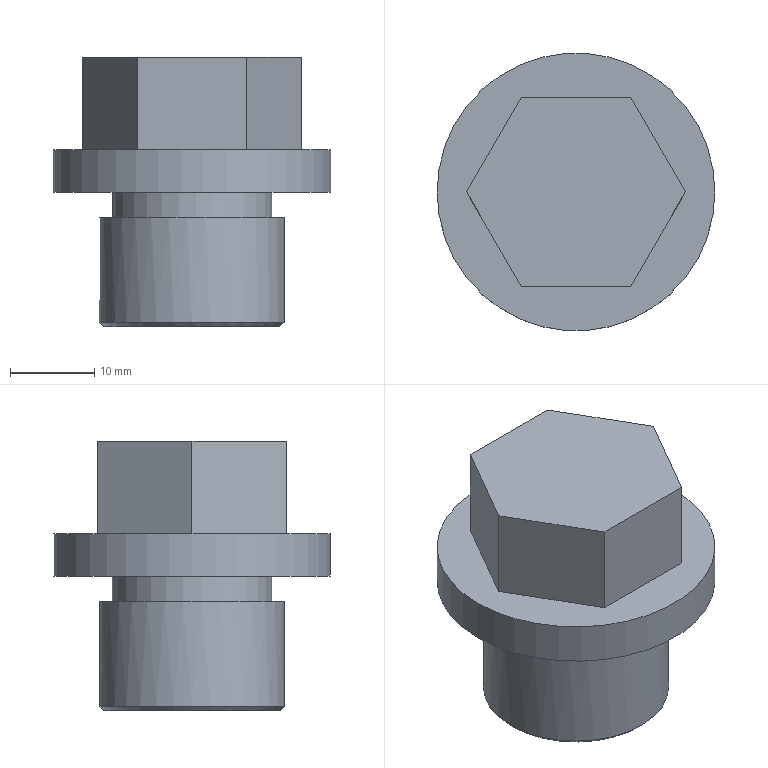Part | NX | features DATUM_CSYS 5, EXTRUDE 4, SKETCH 4, CHAMFER 1 | 1 solid | 15 faces | box 33 x 33 x 32 mm | volume 14890 mm3 | plane 11 | cylinder 3 | cone 1 | commonest cylinder face diameters 19 x1 22 x1 33 x1
STEP:
#1=CARTESIAN_POINT('',(-13.,0.,0.));
#2=VERTEX_POINT('',#1);
#3=CARTESIAN_POINT('',(-6.5,-11.258,0.));
#4=VERTEX_POINT('',#3);
#5=CARTESIAN_POINT('',(-13.,0.,0.));
#6=DIRECTION('',(0.5,-0.866,0.));
#7=VECTOR('',#6,1000.);
#8=LINE('',#5,#7);
#9=EDGE_CURVE('',#2,#4,#8,.T.);
#10=ORIENTED_EDGE('',*,*,#9,.T.);
#11=CARTESIAN_POINT('',(-6.5,-11.258,11.));
#12=VERTEX_POINT('',#11);
#13=CARTESIAN_POINT('',(-6.5,-11.258,11.));
#14=DIRECTION('',(0.,0.,-1.));
#15=VECTOR('',#14,1000.);
#16=LINE('',#13,#15);
#17=EDGE_CURVE('',#12,#4,#16,.T.);
#18=ORIENTED_EDGE('',*,*,#17,.F.);
#19=CARTESIAN_POINT('',(-13.,0.,11.));
#20=VERTEX_POINT('',#19);
#21=CARTESIAN_POINT('',(-13.,0.,11.));
#22=DIRECTION('',(0.5,-0.866,0.));
#23=VECTOR('',#22,1000.);
#24=LINE('',#21,#23);
#25=EDGE_CURVE('',#20,#12,#24,.T.);
#26=ORIENTED_EDGE('',*,*,#25,.F.);
#27=CARTESIAN_POINT('',(-13.,0.,11.));
#28=DIRECTION('',(0.,0.,-1.));
#29=VECTOR('',#28,1000.);
#30=LINE('',#27,#29);
#31=EDGE_CURVE('',#20,#2,#30,.T.);
#32=ORIENTED_EDGE('',*,*,#31,.T.);
#33=EDGE_LOOP('',(#10,#18,#26,#32));
#34=FACE_BOUND('',#33,.T.);
#35=CARTESIAN_POINT('',(-13.,0.,11.));
#36=DIRECTION('',(0.866,0.5,0.));
#37=DIRECTION('',(-0.5,0.866,0.));
#38=AXIS2_PLACEMENT_3D('',#35,#36,#37);
#39=PLANE('',#38);
#40=ADVANCED_FACE('',(#34),#39,.F.);
#41=CARTESIAN_POINT('',(6.5,-11.258,0.));
#42=VERTEX_POINT('',#41);
#43=CARTESIAN_POINT('',(-6.5,-11.258,0.));
#44=DIRECTION('',(1.,0.,0.));
#45=VECTOR('',#44,1000.);
#46=LINE('',#43,#45);
#47=EDGE_CURVE('',#4,#42,#46,.T.);
#48=ORIENTED_EDGE('',*,*,#47,.T.);
#49=CARTESIAN_POINT('',(6.5,-11.258,11.));
#50=VERTEX_POINT('',#49);
#51=CARTESIAN_POINT('',(6.5,-11.258,11.));
#52=DIRECTION('',(0.,0.,-1.));
#53=VECTOR('',#52,1000.);
#54=LINE('',#51,#53);
#55=EDGE_CURVE('',#50,#42,#54,.T.);
#56=ORIENTED_EDGE('',*,*,#55,.F.);
#57=CARTESIAN_POINT('',(-6.5,-11.258,11.));
#58=DIRECTION('',(1.,0.,0.));
#59=VECTOR('',#58,1000.);
#60=LINE('',#57,#59);
#61=EDGE_CURVE('',#12,#50,#60,.T.);
#62=ORIENTED_EDGE('',*,*,#61,.F.);
#63=ORIENTED_EDGE('',*,*,#17,.T.);
#64=EDGE_LOOP('',(#48,#56,#62,#63));
#65=FACE_BOUND('',#64,.T.);
#66=CARTESIAN_POINT('',(-6.5,-11.258,11.));
#67=DIRECTION('',(0.,1.,0.));
#68=DIRECTION('',(-1.,0.,0.));
#69=AXIS2_PLACEMENT_3D('',#66,#67,#68);
#70=PLANE('',#69);
#71=ADVANCED_FACE('',(#65),#70,.F.);
#72=CARTESIAN_POINT('',(13.,0.,0.));
#73=VERTEX_POINT('',#72);
#74=CARTESIAN_POINT('',(6.5,-11.258,0.));
#75=DIRECTION('',(0.5,0.866,0.));
#76=VECTOR('',#75,1000.);
#77=LINE('',#74,#76);
#78=EDGE_CURVE('',#42,#73,#77,.T.);
#79=ORIENTED_EDGE('',*,*,#78,.T.);
#80=CARTESIAN_POINT('',(13.,0.,11.));
#81=VERTEX_POINT('',#80);
#82=CARTESIAN_POINT('',(13.,0.,11.));
#83=DIRECTION('',(0.,0.,-1.));
#84=VECTOR('',#83,1000.);
#85=LINE('',#82,#84);
#86=EDGE_CURVE('',#81,#73,#85,.T.);
#87=ORIENTED_EDGE('',*,*,#86,.F.);
#88=CARTESIAN_POINT('',(6.5,-11.258,11.));
#89=DIRECTION('',(0.5,0.866,0.));
#90=VECTOR('',#89,1000.);
#91=LINE('',#88,#90);
#92=EDGE_CURVE('',#50,#81,#91,.T.);
#93=ORIENTED_EDGE('',*,*,#92,.F.);
#94=ORIENTED_EDGE('',*,*,#55,.T.);
#95=EDGE_LOOP('',(#79,#87,#93,#94));
#96=FACE_BOUND('',#95,.T.);
#97=CARTESIAN_POINT('',(6.5,-11.258,11.));
#98=DIRECTION('',(-0.866,0.5,0.));
#99=DIRECTION('',(-0.5,-0.866,0.));
#100=AXIS2_PLACEMENT_3D('',#97,#98,#99);
#101=PLANE('',#100);
#102=ADVANCED_FACE('',(#96),#101,.F.);
#103=CARTESIAN_POINT('',(6.5,11.258,0.));
#104=VERTEX_POINT('',#103);
#105=CARTESIAN_POINT('',(13.,0.,0.));
#106=DIRECTION('',(-0.5,0.866,0.));
#107=VECTOR('',#106,1000.);
#108=LINE('',#105,#107);
#109=EDGE_CURVE('',#73,#104,#108,.T.);
#110=ORIENTED_EDGE('',*,*,#109,.T.);
#111=CARTESIAN_POINT('',(6.5,11.258,11.));
#112=VERTEX_POINT('',#111);
#113=CARTESIAN_POINT('',(6.5,11.258,11.));
#114=DIRECTION('',(0.,0.,-1.));
#115=VECTOR('',#114,1000.);
#116=LINE('',#113,#115);
#117=EDGE_CURVE('',#112,#104,#116,.T.);
#118=ORIENTED_EDGE('',*,*,#117,.F.);
#119=CARTESIAN_POINT('',(13.,0.,11.));
#120=DIRECTION('',(-0.5,0.866,0.));
#121=VECTOR('',#120,1000.);
#122=LINE('',#119,#121);
#123=EDGE_CURVE('',#81,#112,#122,.T.);
#124=ORIENTED_EDGE('',*,*,#123,.F.);
#125=ORIENTED_EDGE('',*,*,#86,.T.);
#126=EDGE_LOOP('',(#110,#118,#124,#125));
#127=FACE_BOUND('',#126,.T.);
#128=CARTESIAN_POINT('',(13.,0.,11.));
#129=DIRECTION('',(-0.866,-0.5,0.));
#130=DIRECTION('',(0.5,-0.866,0.));
#131=AXIS2_PLACEMENT_3D('',#128,#129,#130);
#132=PLANE('',#131);
#133=ADVANCED_FACE('',(#127),#132,.F.);
#134=CARTESIAN_POINT('',(-6.5,11.258,0.));
#135=VERTEX_POINT('',#134);
#136=CARTESIAN_POINT('',(6.5,11.258,0.));
#137=DIRECTION('',(-1.,0.,0.));
#138=VECTOR('',#137,1000.);
#139=LINE('',#136,#138);
#140=EDGE_CURVE('',#104,#135,#139,.T.);
#141=ORIENTED_EDGE('',*,*,#140,.T.);
#142=CARTESIAN_POINT('',(-6.5,11.258,11.));
#143=VERTEX_POINT('',#142);
#144=CARTESIAN_POINT('',(-6.5,11.258,11.));
#145=DIRECTION('',(0.,0.,-1.));
#146=VECTOR('',#145,1000.);
#147=LINE('',#144,#146);
#148=EDGE_CURVE('',#143,#135,#147,.T.);
#149=ORIENTED_EDGE('',*,*,#148,.F.);
#150=CARTESIAN_POINT('',(6.5,11.258,11.));
#151=DIRECTION('',(-1.,0.,0.));
#152=VECTOR('',#151,1000.);
#153=LINE('',#150,#152);
#154=EDGE_CURVE('',#112,#143,#153,.T.);
#155=ORIENTED_EDGE('',*,*,#154,.F.);
#156=ORIENTED_EDGE('',*,*,#117,.T.);
#157=EDGE_LOOP('',(#141,#149,#155,#156));
#158=FACE_BOUND('',#157,.T.);
#159=CARTESIAN_POINT('',(6.5,11.258,11.));
#160=DIRECTION('',(0.,-1.,0.));
#161=DIRECTION('',(1.,0.,0.));
#162=AXIS2_PLACEMENT_3D('',#159,#160,#161);
#163=PLANE('',#162);
#164=ADVANCED_FACE('',(#158),#163,.F.);
#165=CARTESIAN_POINT('',(-6.5,11.258,0.));
#166=DIRECTION('',(-0.5,-0.866,0.));
#167=VECTOR('',#166,1000.);
#168=LINE('',#165,#167);
#169=EDGE_CURVE('',#135,#2,#168,.T.);
#170=ORIENTED_EDGE('',*,*,#169,.T.);
#171=ORIENTED_EDGE('',*,*,#31,.F.);
#172=CARTESIAN_POINT('',(-6.5,11.258,11.));
#173=DIRECTION('',(-0.5,-0.866,0.));
#174=VECTOR('',#173,1000.);
#175=LINE('',#172,#174);
#176=EDGE_CURVE('',#143,#20,#175,.T.);
#177=ORIENTED_EDGE('',*,*,#176,.F.);
#178=ORIENTED_EDGE('',*,*,#148,.T.);
#179=EDGE_LOOP('',(#170,#171,#177,#178));
#180=FACE_BOUND('',#179,.T.);
#181=CARTESIAN_POINT('',(-6.5,11.258,11.));
#182=DIRECTION('',(0.866,-0.5,0.));
#183=DIRECTION('',(0.5,0.866,0.));
#184=AXIS2_PLACEMENT_3D('',#181,#182,#183);
#185=PLANE('',#184);
#186=ADVANCED_FACE('',(#180),#185,.F.);
#187=ORIENTED_EDGE('',*,*,#25,.T.);
#188=ORIENTED_EDGE('',*,*,#61,.T.);
#189=ORIENTED_EDGE('',*,*,#92,.T.);
#190=ORIENTED_EDGE('',*,*,#123,.T.);
#191=ORIENTED_EDGE('',*,*,#154,.T.);
#192=ORIENTED_EDGE('',*,*,#176,.T.);
#193=EDGE_LOOP('',(#187,#188,#189,#190,#191,#192));
#194=FACE_BOUND('',#193,.T.);
#195=CARTESIAN_POINT('',(0.,0.,11.));
#196=DIRECTION('',(0.,0.,1.));
#197=DIRECTION('',(1.,0.,0.));
#198=AXIS2_PLACEMENT_3D('',#195,#196,#197);
#199=PLANE('',#198);
#200=ADVANCED_FACE('',(#194),#199,.T.);
#201=CARTESIAN_POINT('',(16.5,0.,0.));
#202=VERTEX_POINT('',#201);
#203=CARTESIAN_POINT('',(0.,0.,0.));
#204=DIRECTION('',(0.,0.,1.));
#205=DIRECTION('',(1.,0.,0.));
#206=AXIS2_PLACEMENT_3D('',#203,#204,#205);
#207=CIRCLE('',#206,16.5);
#208=EDGE_CURVE('',#202,#202,#207,.T.);
#209=ORIENTED_EDGE('',*,*,#208,.T.);
#210=EDGE_LOOP('',(#209));
#211=FACE_BOUND('',#210,.T.);
#212=ORIENTED_EDGE('',*,*,#9,.F.);
#213=ORIENTED_EDGE('',*,*,#169,.F.);
#214=ORIENTED_EDGE('',*,*,#140,.F.);
#215=ORIENTED_EDGE('',*,*,#109,.F.);
#216=ORIENTED_EDGE('',*,*,#78,.F.);
#217=ORIENTED_EDGE('',*,*,#47,.F.);
#218=EDGE_LOOP('',(#212,#213,#214,#215,#216,#217));
#219=FACE_BOUND('',#218,.T.);
#220=CARTESIAN_POINT('',(0.,0.,0.));
#221=DIRECTION('',(0.,0.,1.));
#222=DIRECTION('',(1.,0.,0.));
#223=AXIS2_PLACEMENT_3D('',#220,#221,#222);
#224=PLANE('',#223);
#225=ADVANCED_FACE('',(#211,#219),#224,.T.);
#226=CARTESIAN_POINT('',(16.5,0.,-5.));
#227=VERTEX_POINT('',#226);
#228=CARTESIAN_POINT('',(0.,0.,-5.));
#229=DIRECTION('',(0.,0.,1.));
#230=DIRECTION('',(1.,0.,0.));
#231=AXIS2_PLACEMENT_3D('',#228,#229,#230);
#232=CIRCLE('',#231,16.5);
#233=EDGE_CURVE('',#227,#227,#232,.T.);
#234=ORIENTED_EDGE('',*,*,#233,.T.);
#235=EDGE_LOOP('',(#234));
#236=FACE_BOUND('',#235,.T.);
#237=ORIENTED_EDGE('',*,*,#208,.F.);
#238=EDGE_LOOP('',(#237));
#239=FACE_BOUND('',#238,.T.);
#240=CARTESIAN_POINT('',(0.,0.,-5.));
#241=DIRECTION('',(0.,0.,1.));
#242=DIRECTION('',(1.,0.,0.));
#243=AXIS2_PLACEMENT_3D('',#240,#241,#242);
#244=CYLINDRICAL_SURFACE('',#243,16.5);
#245=ADVANCED_FACE('',(#236,#239),#244,.T.);
#246=CARTESIAN_POINT('',(9.5,0.,-5.));
#247=VERTEX_POINT('',#246);
#248=CARTESIAN_POINT('',(0.,0.,-5.));
#249=DIRECTION('',(0.,0.,-1.));
#250=DIRECTION('',(1.,0.,0.));
#251=AXIS2_PLACEMENT_3D('',#248,#249,#250);
#252=CIRCLE('',#251,9.5);
#253=EDGE_CURVE('',#247,#247,#252,.T.);
#254=ORIENTED_EDGE('',*,*,#253,.F.);
#255=EDGE_LOOP('',(#254));
#256=FACE_BOUND('',#255,.T.);
#257=ORIENTED_EDGE('',*,*,#233,.F.);
#258=EDGE_LOOP('',(#257));
#259=FACE_BOUND('',#258,.T.);
#260=CARTESIAN_POINT('',(0.,0.,-5.));
#261=DIRECTION('',(0.,0.,1.));
#262=DIRECTION('',(1.,0.,0.));
#263=AXIS2_PLACEMENT_3D('',#260,#261,#262);
#264=PLANE('',#263);
#265=ADVANCED_FACE('',(#256,#259),#264,.F.);
#266=CARTESIAN_POINT('',(9.5,0.,-8.));
#267=VERTEX_POINT('',#266);
#268=CARTESIAN_POINT('',(0.,0.,-8.));
#269=DIRECTION('',(0.,0.,-1.));
#270=DIRECTION('',(1.,0.,0.));
#271=AXIS2_PLACEMENT_3D('',#268,#269,#270);
#272=CIRCLE('',#271,9.5);
#273=EDGE_CURVE('',#267,#267,#272,.T.);
#274=ORIENTED_EDGE('',*,*,#273,.F.);
#275=EDGE_LOOP('',(#274));
#276=FACE_BOUND('',#275,.T.);
#277=ORIENTED_EDGE('',*,*,#253,.T.);
#278=EDGE_LOOP('',(#277));
#279=FACE_BOUND('',#278,.T.);
#280=CARTESIAN_POINT('',(0.,0.,-8.));
#281=DIRECTION('',(0.,0.,1.));
#282=DIRECTION('',(1.,0.,0.));
#283=AXIS2_PLACEMENT_3D('',#280,#281,#282);
#284=CYLINDRICAL_SURFACE('',#283,9.5);
#285=ADVANCED_FACE('',(#276,#279),#284,.T.);
#286=CARTESIAN_POINT('',(-11.,0.,-20.5));
#287=VERTEX_POINT('',#286);
#288=CARTESIAN_POINT('',(0.,0.,-20.5));
#289=DIRECTION('',(0.,0.,-1.));
#290=DIRECTION('',(-1.,0.,0.));
#291=AXIS2_PLACEMENT_3D('',#288,#289,#290);
#292=CIRCLE('',#291,11.);
#293=EDGE_CURVE('',#287,#287,#292,.F.);
#294=ORIENTED_EDGE('',*,*,#293,.T.);
#295=EDGE_LOOP('',(#294));
#296=FACE_BOUND('',#295,.T.);
#297=CARTESIAN_POINT('',(11.,0.,-8.));
#298=VERTEX_POINT('',#297);
#299=CARTESIAN_POINT('',(0.,0.,-8.));
#300=DIRECTION('',(0.,0.,-1.));
#301=DIRECTION('',(1.,0.,0.));
#302=AXIS2_PLACEMENT_3D('',#299,#300,#301);
#303=CIRCLE('',#302,11.);
#304=EDGE_CURVE('',#298,#298,#303,.T.);
#305=ORIENTED_EDGE('',*,*,#304,.T.);
#306=EDGE_LOOP('',(#305));
#307=FACE_BOUND('',#306,.T.);
#308=CARTESIAN_POINT('',(0.,0.,-21.));
#309=DIRECTION('',(0.,0.,1.));
#310=DIRECTION('',(1.,0.,0.));
#311=AXIS2_PLACEMENT_3D('',#308,#309,#310);
#312=CYLINDRICAL_SURFACE('',#311,11.);
#313=ADVANCED_FACE('',(#296,#307),#312,.T.);
#314=CARTESIAN_POINT('',(-10.5,0.,-21.));
#315=VERTEX_POINT('',#314);
#316=CARTESIAN_POINT('',(0.,0.,-21.));
#317=DIRECTION('',(0.,0.,-1.));
#318=DIRECTION('',(-1.,0.,0.));
#319=AXIS2_PLACEMENT_3D('',#316,#317,#318);
#320=CIRCLE('',#319,10.5);
#321=EDGE_CURVE('',#315,#315,#320,.T.);
#322=ORIENTED_EDGE('',*,*,#321,.T.);
#323=EDGE_LOOP('',(#322));
#324=FACE_BOUND('',#323,.T.);
#325=CARTESIAN_POINT('',(0.,0.,-21.));
#326=DIRECTION('',(0.,0.,-1.));
#327=DIRECTION('',(-1.,0.,0.));
#328=AXIS2_PLACEMENT_3D('',#325,#326,#327);
#329=PLANE('',#328);
#330=ADVANCED_FACE('',(#324),#329,.T.);
#331=ORIENTED_EDGE('',*,*,#273,.T.);
#332=EDGE_LOOP('',(#331));
#333=FACE_BOUND('',#332,.T.);
#334=ORIENTED_EDGE('',*,*,#304,.F.);
#335=EDGE_LOOP('',(#334));
#336=FACE_BOUND('',#335,.T.);
#337=CARTESIAN_POINT('',(0.,0.,-8.));
#338=DIRECTION('',(0.,0.,-1.));
#339=DIRECTION('',(-1.,0.,0.));
#340=AXIS2_PLACEMENT_3D('',#337,#338,#339);
#341=PLANE('',#340);
#342=ADVANCED_FACE('',(#333,#336),#341,.F.);
#343=ORIENTED_EDGE('',*,*,#293,.F.);
#344=EDGE_LOOP('',(#343));
#345=FACE_BOUND('',#344,.T.);
#346=ORIENTED_EDGE('',*,*,#321,.F.);
#347=EDGE_LOOP('',(#346));
#348=FACE_BOUND('',#347,.T.);
#349=CARTESIAN_POINT('',(0.,0.,-21.));
#350=DIRECTION('',(0.,0.,1.));
#351=DIRECTION('',(1.,0.,0.));
#352=AXIS2_PLACEMENT_3D('',#349,#350,#351);
#353=CONICAL_SURFACE('',#352,10.5,0.7854);
#354=ADVANCED_FACE('',(#345,#348),#353,.T.);
#355=CLOSED_SHELL('',(#40,#71,#102,#133,#164,#186,#200,#225,#245,#265,#285,#313,#330,#342,#354));
#356=MANIFOLD_SOLID_BREP('',#355);
#357=(LENGTH_UNIT()NAMED_UNIT(*)SI_UNIT(.MILLI.,.METRE.));
#358=UNCERTAINTY_MEASURE_WITH_UNIT(LENGTH_MEASURE(0.00001),#357,'','');
#359=(NAMED_UNIT(*)PLANE_ANGLE_UNIT()SI_UNIT($,.RADIAN.));
#360=(NAMED_UNIT(*)SI_UNIT($,.STERADIAN.)SOLID_ANGLE_UNIT());
#361=(GEOMETRIC_REPRESENTATION_CONTEXT(3)GLOBAL_UNCERTAINTY_ASSIGNED_CONTEXT((#358))GLOBAL_UNIT_ASSIGNED_CONTEXT((#357,#359,#360))REPRESENTATION_CONTEXT('',''));
#362=ADVANCED_BREP_SHAPE_REPRESENTATION('',(#356),#361);